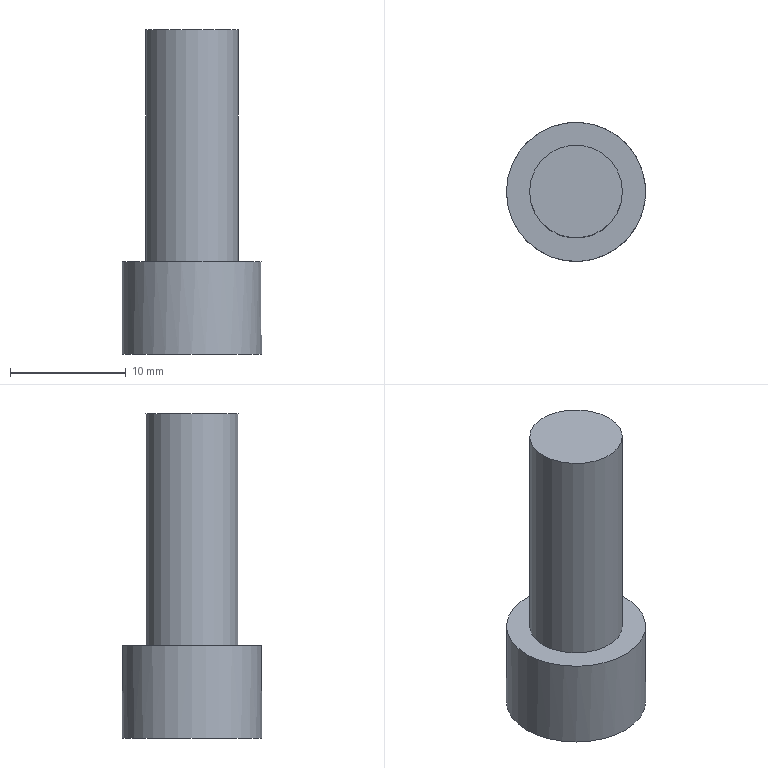Part | NX | features solid 2 | 1 solid | 12 faces | box 12 x 12 x 28 mm | volume 1740 mm3 | plane 10 | cylinder 2 | commonest cylinder face diameters 8 x1 12 x1
STEP:
#1=CARTESIAN_POINT('',(22.2,45.152,340.));
#2=VERTEX_POINT('',#1);
#3=CARTESIAN_POINT('',(19.,43.305,340.));
#4=VERTEX_POINT('',#3);
#5=CARTESIAN_POINT('',(20.6,44.229,340.));
#6=DIRECTION('',(-0.866,-0.5,0.));
#7=VECTOR('',#6,1000.);
#8=LINE('',#5,#7);
#9=EDGE_CURVE('',#2,#4,#8,.T.);
#10=ORIENTED_EDGE('',*,*,#9,.F.);
#11=CARTESIAN_POINT('',(22.2,48.848,340.));
#12=VERTEX_POINT('',#11);
#13=CARTESIAN_POINT('',(22.2,47.,340.));
#14=DIRECTION('',(0.,-1.,0.));
#15=VECTOR('',#14,1000.);
#16=LINE('',#13,#15);
#17=EDGE_CURVE('',#12,#2,#16,.T.);
#18=ORIENTED_EDGE('',*,*,#17,.F.);
#19=CARTESIAN_POINT('',(19.,50.695,340.));
#20=VERTEX_POINT('',#19);
#21=CARTESIAN_POINT('',(20.6,49.771,340.));
#22=DIRECTION('',(0.866,-0.5,0.));
#23=VECTOR('',#22,1000.);
#24=LINE('',#21,#23);
#25=EDGE_CURVE('',#20,#12,#24,.T.);
#26=ORIENTED_EDGE('',*,*,#25,.F.);
#27=CARTESIAN_POINT('',(15.8,48.848,340.));
#28=VERTEX_POINT('',#27);
#29=CARTESIAN_POINT('',(17.4,49.771,340.));
#30=DIRECTION('',(0.866,0.5,0.));
#31=VECTOR('',#30,1000.);
#32=LINE('',#29,#31);
#33=EDGE_CURVE('',#28,#20,#32,.T.);
#34=ORIENTED_EDGE('',*,*,#33,.F.);
#35=CARTESIAN_POINT('',(15.8,45.152,340.));
#36=VERTEX_POINT('',#35);
#37=CARTESIAN_POINT('',(15.8,47.,340.));
#38=DIRECTION('',(0.,1.,0.));
#39=VECTOR('',#38,1000.);
#40=LINE('',#37,#39);
#41=EDGE_CURVE('',#36,#28,#40,.T.);
#42=ORIENTED_EDGE('',*,*,#41,.F.);
#43=CARTESIAN_POINT('',(17.4,44.229,340.));
#44=DIRECTION('',(-0.866,0.5,0.));
#45=VECTOR('',#44,1000.);
#46=LINE('',#43,#45);
#47=EDGE_CURVE('',#4,#36,#46,.T.);
#48=ORIENTED_EDGE('',*,*,#47,.F.);
#49=EDGE_LOOP('',(#10,#18,#26,#34,#42,#48));
#50=FACE_BOUND('',#49,.T.);
#51=CARTESIAN_POINT('',(25.,47.,340.));
#52=VERTEX_POINT('',#51);
#53=CARTESIAN_POINT('',(19.,47.,340.));
#54=DIRECTION('',(0.,0.,1.));
#55=DIRECTION('',(1.,0.,0.));
#56=AXIS2_PLACEMENT_3D('',#53,#54,#55);
#57=CIRCLE('',#56,6.);
#58=EDGE_CURVE('',#52,#52,#57,.T.);
#59=ORIENTED_EDGE('',*,*,#58,.F.);
#60=EDGE_LOOP('',(#59));
#61=FACE_BOUND('',#60,.T.);
#62=CARTESIAN_POINT('',(19.,47.,340.));
#63=DIRECTION('',(0.,0.,-1.));
#64=DIRECTION('',(-1.,0.,0.));
#65=AXIS2_PLACEMENT_3D('',#62,#63,#64);
#66=PLANE('',#65);
#67=ADVANCED_FACE('',(#50,#61),#66,.T.);
#68=CARTESIAN_POINT('',(23.,47.,348.));
#69=VERTEX_POINT('',#68);
#70=CARTESIAN_POINT('',(19.,47.,348.));
#71=DIRECTION('',(0.,0.,1.));
#72=DIRECTION('',(1.,0.,0.));
#73=AXIS2_PLACEMENT_3D('',#70,#71,#72);
#74=CIRCLE('',#73,4.);
#75=EDGE_CURVE('',#69,#69,#74,.T.);
#76=ORIENTED_EDGE('',*,*,#75,.F.);
#77=EDGE_LOOP('',(#76));
#78=FACE_BOUND('',#77,.T.);
#79=CARTESIAN_POINT('',(13.,47.,348.));
#80=VERTEX_POINT('',#79);
#81=CARTESIAN_POINT('',(19.,47.,348.));
#82=DIRECTION('',(0.,0.,-1.));
#83=DIRECTION('',(-1.,0.,0.));
#84=AXIS2_PLACEMENT_3D('',#81,#82,#83);
#85=CIRCLE('',#84,6.);
#86=EDGE_CURVE('',#80,#80,#85,.T.);
#87=ORIENTED_EDGE('',*,*,#86,.F.);
#88=EDGE_LOOP('',(#87));
#89=FACE_BOUND('',#88,.T.);
#90=CARTESIAN_POINT('',(19.,47.,348.));
#91=DIRECTION('',(0.,0.,1.));
#92=DIRECTION('',(1.,0.,0.));
#93=AXIS2_PLACEMENT_3D('',#90,#91,#92);
#94=PLANE('',#93);
#95=ADVANCED_FACE('',(#78,#89),#94,.T.);
#96=ORIENTED_EDGE('',*,*,#58,.T.);
#97=EDGE_LOOP('',(#96));
#98=FACE_BOUND('',#97,.T.);
#99=ORIENTED_EDGE('',*,*,#86,.T.);
#100=EDGE_LOOP('',(#99));
#101=FACE_BOUND('',#100,.T.);
#102=CARTESIAN_POINT('',(19.,47.,348.));
#103=DIRECTION('',(0.,0.,-1.));
#104=DIRECTION('',(-1.,0.,0.));
#105=AXIS2_PLACEMENT_3D('',#102,#103,#104);
#106=CYLINDRICAL_SURFACE('',#105,6.);
#107=ADVANCED_FACE('',(#98,#101),#106,.T.);
#108=ORIENTED_EDGE('',*,*,#9,.T.);
#109=CARTESIAN_POINT('',(19.,43.305,344.8));
#110=VERTEX_POINT('',#109);
#111=CARTESIAN_POINT('',(19.,43.305,344.8));
#112=DIRECTION('',(0.,0.,-1.));
#113=VECTOR('',#112,1000.);
#114=LINE('',#111,#113);
#115=EDGE_CURVE('',#110,#4,#114,.T.);
#116=ORIENTED_EDGE('',*,*,#115,.F.);
#117=CARTESIAN_POINT('',(22.2,45.152,344.8));
#118=VERTEX_POINT('',#117);
#119=CARTESIAN_POINT('',(22.2,45.152,344.8));
#120=DIRECTION('',(-0.866,-0.5,0.));
#121=VECTOR('',#120,1000.);
#122=LINE('',#119,#121);
#123=EDGE_CURVE('',#118,#110,#122,.T.);
#124=ORIENTED_EDGE('',*,*,#123,.F.);
#125=CARTESIAN_POINT('',(22.2,45.152,344.8));
#126=DIRECTION('',(0.,0.,-1.));
#127=VECTOR('',#126,1000.);
#128=LINE('',#125,#127);
#129=EDGE_CURVE('',#118,#2,#128,.T.);
#130=ORIENTED_EDGE('',*,*,#129,.T.);
#131=EDGE_LOOP('',(#108,#116,#124,#130));
#132=FACE_BOUND('',#131,.T.);
#133=CARTESIAN_POINT('',(20.6,44.229,340.8));
#134=DIRECTION('',(0.5,-0.866,0.));
#135=DIRECTION('',(0.866,0.5,0.));
#136=AXIS2_PLACEMENT_3D('',#133,#134,#135);
#137=PLANE('',#136);
#138=ADVANCED_FACE('',(#132),#137,.F.);
#139=ORIENTED_EDGE('',*,*,#17,.T.);
#140=ORIENTED_EDGE('',*,*,#129,.F.);
#141=CARTESIAN_POINT('',(22.2,48.848,344.8));
#142=VERTEX_POINT('',#141);
#143=CARTESIAN_POINT('',(22.2,48.848,344.8));
#144=DIRECTION('',(0.,-1.,0.));
#145=VECTOR('',#144,1000.);
#146=LINE('',#143,#145);
#147=EDGE_CURVE('',#142,#118,#146,.T.);
#148=ORIENTED_EDGE('',*,*,#147,.F.);
#149=CARTESIAN_POINT('',(22.2,48.848,344.8));
#150=DIRECTION('',(0.,0.,-1.));
#151=VECTOR('',#150,1000.);
#152=LINE('',#149,#151);
#153=EDGE_CURVE('',#142,#12,#152,.T.);
#154=ORIENTED_EDGE('',*,*,#153,.T.);
#155=EDGE_LOOP('',(#139,#140,#148,#154));
#156=FACE_BOUND('',#155,.T.);
#157=CARTESIAN_POINT('',(22.2,47.,340.8));
#158=DIRECTION('',(1.,0.,0.));
#159=DIRECTION('',(0.,0.,-1.));
#160=AXIS2_PLACEMENT_3D('',#157,#158,#159);
#161=PLANE('',#160);
#162=ADVANCED_FACE('',(#156),#161,.F.);
#163=ORIENTED_EDGE('',*,*,#25,.T.);
#164=ORIENTED_EDGE('',*,*,#153,.F.);
#165=CARTESIAN_POINT('',(19.,50.695,344.8));
#166=VERTEX_POINT('',#165);
#167=CARTESIAN_POINT('',(19.,50.695,344.8));
#168=DIRECTION('',(0.866,-0.5,0.));
#169=VECTOR('',#168,1000.);
#170=LINE('',#167,#169);
#171=EDGE_CURVE('',#166,#142,#170,.T.);
#172=ORIENTED_EDGE('',*,*,#171,.F.);
#173=CARTESIAN_POINT('',(19.,50.695,344.8));
#174=DIRECTION('',(0.,0.,-1.));
#175=VECTOR('',#174,1000.);
#176=LINE('',#173,#175);
#177=EDGE_CURVE('',#166,#20,#176,.T.);
#178=ORIENTED_EDGE('',*,*,#177,.T.);
#179=EDGE_LOOP('',(#163,#164,#172,#178));
#180=FACE_BOUND('',#179,.T.);
#181=CARTESIAN_POINT('',(20.6,49.771,340.8));
#182=DIRECTION('',(0.5,0.866,0.));
#183=DIRECTION('',(-0.866,0.5,0.));
#184=AXIS2_PLACEMENT_3D('',#181,#182,#183);
#185=PLANE('',#184);
#186=ADVANCED_FACE('',(#180),#185,.F.);
#187=ORIENTED_EDGE('',*,*,#33,.T.);
#188=ORIENTED_EDGE('',*,*,#177,.F.);
#189=CARTESIAN_POINT('',(15.8,48.848,344.8));
#190=VERTEX_POINT('',#189);
#191=CARTESIAN_POINT('',(15.8,48.848,344.8));
#192=DIRECTION('',(0.866,0.5,0.));
#193=VECTOR('',#192,1000.);
#194=LINE('',#191,#193);
#195=EDGE_CURVE('',#190,#166,#194,.T.);
#196=ORIENTED_EDGE('',*,*,#195,.F.);
#197=CARTESIAN_POINT('',(15.8,48.848,344.8));
#198=DIRECTION('',(0.,0.,-1.));
#199=VECTOR('',#198,1000.);
#200=LINE('',#197,#199);
#201=EDGE_CURVE('',#190,#28,#200,.T.);
#202=ORIENTED_EDGE('',*,*,#201,.T.);
#203=EDGE_LOOP('',(#187,#188,#196,#202));
#204=FACE_BOUND('',#203,.T.);
#205=CARTESIAN_POINT('',(17.4,49.771,340.8));
#206=DIRECTION('',(-0.5,0.866,0.));
#207=DIRECTION('',(-0.866,-0.5,0.));
#208=AXIS2_PLACEMENT_3D('',#205,#206,#207);
#209=PLANE('',#208);
#210=ADVANCED_FACE('',(#204),#209,.F.);
#211=ORIENTED_EDGE('',*,*,#41,.T.);
#212=ORIENTED_EDGE('',*,*,#201,.F.);
#213=CARTESIAN_POINT('',(15.8,45.152,344.8));
#214=VERTEX_POINT('',#213);
#215=CARTESIAN_POINT('',(15.8,45.152,344.8));
#216=DIRECTION('',(0.,1.,0.));
#217=VECTOR('',#216,1000.);
#218=LINE('',#215,#217);
#219=EDGE_CURVE('',#214,#190,#218,.T.);
#220=ORIENTED_EDGE('',*,*,#219,.F.);
#221=CARTESIAN_POINT('',(15.8,45.152,344.8));
#222=DIRECTION('',(0.,0.,-1.));
#223=VECTOR('',#222,1000.);
#224=LINE('',#221,#223);
#225=EDGE_CURVE('',#214,#36,#224,.T.);
#226=ORIENTED_EDGE('',*,*,#225,.T.);
#227=EDGE_LOOP('',(#211,#212,#220,#226));
#228=FACE_BOUND('',#227,.T.);
#229=CARTESIAN_POINT('',(15.8,47.,340.8));
#230=DIRECTION('',(-1.,0.,0.));
#231=DIRECTION('',(0.,-1.,0.));
#232=AXIS2_PLACEMENT_3D('',#229,#230,#231);
#233=PLANE('',#232);
#234=ADVANCED_FACE('',(#228),#233,.F.);
#235=ORIENTED_EDGE('',*,*,#47,.T.);
#236=ORIENTED_EDGE('',*,*,#225,.F.);
#237=CARTESIAN_POINT('',(19.,43.305,344.8));
#238=DIRECTION('',(-0.866,0.5,0.));
#239=VECTOR('',#238,1000.);
#240=LINE('',#237,#239);
#241=EDGE_CURVE('',#110,#214,#240,.T.);
#242=ORIENTED_EDGE('',*,*,#241,.F.);
#243=ORIENTED_EDGE('',*,*,#115,.T.);
#244=EDGE_LOOP('',(#235,#236,#242,#243));
#245=FACE_BOUND('',#244,.T.);
#246=CARTESIAN_POINT('',(17.4,44.229,340.8));
#247=DIRECTION('',(-0.5,-0.866,0.));
#248=DIRECTION('',(0.866,-0.5,0.));
#249=AXIS2_PLACEMENT_3D('',#246,#247,#248);
#250=PLANE('',#249);
#251=ADVANCED_FACE('',(#245),#250,.F.);
#252=ORIENTED_EDGE('',*,*,#241,.T.);
#253=ORIENTED_EDGE('',*,*,#219,.T.);
#254=ORIENTED_EDGE('',*,*,#195,.T.);
#255=ORIENTED_EDGE('',*,*,#171,.T.);
#256=ORIENTED_EDGE('',*,*,#147,.T.);
#257=ORIENTED_EDGE('',*,*,#123,.T.);
#258=EDGE_LOOP('',(#252,#253,#254,#255,#256,#257));
#259=FACE_BOUND('',#258,.T.);
#260=CARTESIAN_POINT('',(19.,47.,344.8));
#261=DIRECTION('',(0.,0.,1.));
#262=DIRECTION('',(1.,0.,0.));
#263=AXIS2_PLACEMENT_3D('',#260,#261,#262);
#264=PLANE('',#263);
#265=ADVANCED_FACE('',(#259),#264,.F.);
#266=CARTESIAN_POINT('',(15.,47.,368.));
#267=VERTEX_POINT('',#266);
#268=CARTESIAN_POINT('',(19.,47.,368.));
#269=DIRECTION('',(0.,0.,-1.));
#270=DIRECTION('',(-1.,0.,0.));
#271=AXIS2_PLACEMENT_3D('',#268,#269,#270);
#272=CIRCLE('',#271,4.);
#273=EDGE_CURVE('',#267,#267,#272,.T.);
#274=ORIENTED_EDGE('',*,*,#273,.F.);
#275=EDGE_LOOP('',(#274));
#276=FACE_BOUND('',#275,.T.);
#277=CARTESIAN_POINT('',(19.,47.,368.));
#278=DIRECTION('',(0.,0.,1.));
#279=DIRECTION('',(1.,0.,0.));
#280=AXIS2_PLACEMENT_3D('',#277,#278,#279);
#281=PLANE('',#280);
#282=ADVANCED_FACE('',(#276),#281,.T.);
#283=ORIENTED_EDGE('',*,*,#273,.T.);
#284=EDGE_LOOP('',(#283));
#285=FACE_BOUND('',#284,.T.);
#286=ORIENTED_EDGE('',*,*,#75,.T.);
#287=EDGE_LOOP('',(#286));
#288=FACE_BOUND('',#287,.T.);
#289=CARTESIAN_POINT('',(19.,47.,348.));
#290=DIRECTION('',(0.,0.,1.));
#291=DIRECTION('',(1.,0.,0.));
#292=AXIS2_PLACEMENT_3D('',#289,#290,#291);
#293=CYLINDRICAL_SURFACE('',#292,4.);
#294=ADVANCED_FACE('',(#285,#288),#293,.T.);
#295=CLOSED_SHELL('',(#67,#95,#107,#138,#162,#186,#210,#234,#251,#265,#282,#294));
#296=MANIFOLD_SOLID_BREP('',#295);
#297=(LENGTH_UNIT()NAMED_UNIT(*)SI_UNIT(.MILLI.,.METRE.));
#298=UNCERTAINTY_MEASURE_WITH_UNIT(LENGTH_MEASURE(0.00001),#297,'','');
#299=(NAMED_UNIT(*)PLANE_ANGLE_UNIT()SI_UNIT($,.RADIAN.));
#300=(NAMED_UNIT(*)SI_UNIT($,.STERADIAN.)SOLID_ANGLE_UNIT());
#301=(GEOMETRIC_REPRESENTATION_CONTEXT(3)GLOBAL_UNCERTAINTY_ASSIGNED_CONTEXT((#298))GLOBAL_UNIT_ASSIGNED_CONTEXT((#297,#299,#300))REPRESENTATION_CONTEXT('',''));
#302=ADVANCED_BREP_SHAPE_REPRESENTATION('',(#296),#301);